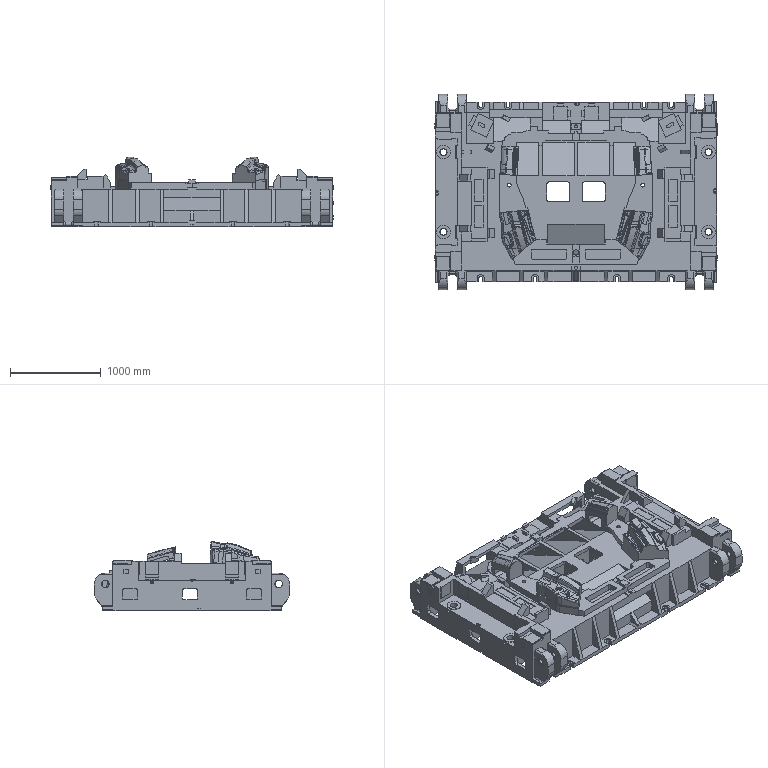Part | NX | features solid 2 | 1 solid | 2490 faces | box 3110 x 2150 x 765.026 mm | volume 1004190400 mm3 | plane 1491 | spline 517 | cylinder 474 | torus 8 | commonest cylinder face diameters 40 x328 83 x48 30 x18 79 x16 80 x12 200 x8